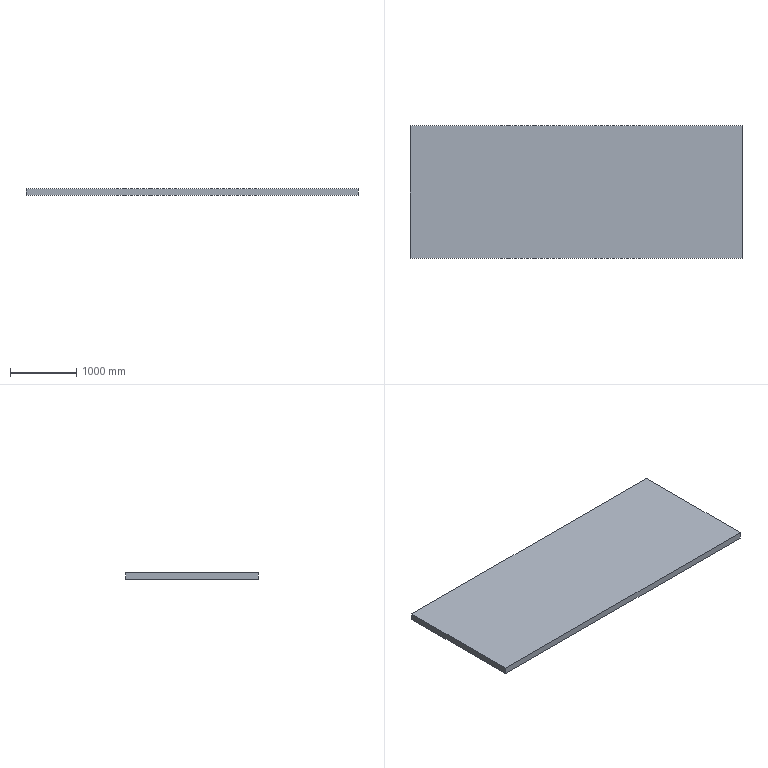Part | SolidWorks | features Extrusion 1 | 1 solid | 6 faces | box 5000 x 2000 x 100 mm | volume 1000000000 mm3 | plane 6
STEP:
#1=CARTESIAN_POINT('',(0.,2000.,0.));
#2=VERTEX_POINT('',#1);
#3=CARTESIAN_POINT('',(0.,0.,0.));
#4=VERTEX_POINT('',#3);
#5=CARTESIAN_POINT('',(0.,0.,0.));
#6=DIRECTION('',(0.,-1.,0.));
#7=VECTOR('',#6,1000.);
#8=LINE('',#5,#7);
#9=EDGE_CURVE('',#2,#4,#8,.T.);
#10=ORIENTED_EDGE('',*,*,#9,.T.);
#11=CARTESIAN_POINT('',(0.,0.,100.));
#12=VERTEX_POINT('',#11);
#13=CARTESIAN_POINT('',(0.,0.,100.));
#14=DIRECTION('',(0.,0.,-1.));
#15=VECTOR('',#14,1000.);
#16=LINE('',#13,#15);
#17=EDGE_CURVE('',#12,#4,#16,.T.);
#18=ORIENTED_EDGE('',*,*,#17,.F.);
#19=CARTESIAN_POINT('',(0.,2000.,100.));
#20=VERTEX_POINT('',#19);
#21=CARTESIAN_POINT('',(0.,0.,100.));
#22=DIRECTION('',(0.,-1.,0.));
#23=VECTOR('',#22,1000.);
#24=LINE('',#21,#23);
#25=EDGE_CURVE('',#20,#12,#24,.T.);
#26=ORIENTED_EDGE('',*,*,#25,.F.);
#27=CARTESIAN_POINT('',(0.,2000.,100.));
#28=DIRECTION('',(0.,0.,-1.));
#29=VECTOR('',#28,1000.);
#30=LINE('',#27,#29);
#31=EDGE_CURVE('',#20,#2,#30,.T.);
#32=ORIENTED_EDGE('',*,*,#31,.T.);
#33=EDGE_LOOP('',(#10,#18,#26,#32));
#34=FACE_OUTER_BOUND('',#33,.T.);
#35=CARTESIAN_POINT('',(0.,0.,100.));
#36=DIRECTION('',(1.,0.,0.));
#37=DIRECTION('',(0.,0.,-1.));
#38=AXIS2_PLACEMENT_3D('',#35,#36,#37);
#39=PLANE('',#38);
#40=ADVANCED_FACE('',(#34),#39,.F.);
#41=CARTESIAN_POINT('',(5000.,0.,0.));
#42=VERTEX_POINT('',#41);
#43=CARTESIAN_POINT('',(0.,0.,0.));
#44=DIRECTION('',(1.,0.,0.));
#45=VECTOR('',#44,1000.);
#46=LINE('',#43,#45);
#47=EDGE_CURVE('',#4,#42,#46,.T.);
#48=ORIENTED_EDGE('',*,*,#47,.T.);
#49=CARTESIAN_POINT('',(5000.,0.,100.));
#50=VERTEX_POINT('',#49);
#51=CARTESIAN_POINT('',(5000.,0.,100.));
#52=DIRECTION('',(0.,0.,-1.));
#53=VECTOR('',#52,1000.);
#54=LINE('',#51,#53);
#55=EDGE_CURVE('',#50,#42,#54,.T.);
#56=ORIENTED_EDGE('',*,*,#55,.F.);
#57=CARTESIAN_POINT('',(0.,0.,100.));
#58=DIRECTION('',(1.,0.,0.));
#59=VECTOR('',#58,1000.);
#60=LINE('',#57,#59);
#61=EDGE_CURVE('',#12,#50,#60,.T.);
#62=ORIENTED_EDGE('',*,*,#61,.F.);
#63=ORIENTED_EDGE('',*,*,#17,.T.);
#64=EDGE_LOOP('',(#48,#56,#62,#63));
#65=FACE_OUTER_BOUND('',#64,.T.);
#66=CARTESIAN_POINT('',(0.,0.,100.));
#67=DIRECTION('',(0.,1.,0.));
#68=DIRECTION('',(0.,0.,1.));
#69=AXIS2_PLACEMENT_3D('',#66,#67,#68);
#70=PLANE('',#69);
#71=ADVANCED_FACE('',(#65),#70,.F.);
#72=CARTESIAN_POINT('',(5000.,2000.,0.));
#73=VERTEX_POINT('',#72);
#74=CARTESIAN_POINT('',(5000.,0.,0.));
#75=DIRECTION('',(0.,1.,0.));
#76=VECTOR('',#75,1000.);
#77=LINE('',#74,#76);
#78=EDGE_CURVE('',#42,#73,#77,.T.);
#79=ORIENTED_EDGE('',*,*,#78,.T.);
#80=CARTESIAN_POINT('',(5000.,2000.,100.));
#81=VERTEX_POINT('',#80);
#82=CARTESIAN_POINT('',(5000.,2000.,100.));
#83=DIRECTION('',(0.,0.,-1.));
#84=VECTOR('',#83,1000.);
#85=LINE('',#82,#84);
#86=EDGE_CURVE('',#81,#73,#85,.T.);
#87=ORIENTED_EDGE('',*,*,#86,.F.);
#88=CARTESIAN_POINT('',(5000.,0.,100.));
#89=DIRECTION('',(0.,1.,0.));
#90=VECTOR('',#89,1000.);
#91=LINE('',#88,#90);
#92=EDGE_CURVE('',#50,#81,#91,.T.);
#93=ORIENTED_EDGE('',*,*,#92,.F.);
#94=ORIENTED_EDGE('',*,*,#55,.T.);
#95=EDGE_LOOP('',(#79,#87,#93,#94));
#96=FACE_OUTER_BOUND('',#95,.T.);
#97=CARTESIAN_POINT('',(5000.,0.,100.));
#98=DIRECTION('',(-1.,0.,0.));
#99=DIRECTION('',(0.,0.,1.));
#100=AXIS2_PLACEMENT_3D('',#97,#98,#99);
#101=PLANE('',#100);
#102=ADVANCED_FACE('',(#96),#101,.F.);
#103=CARTESIAN_POINT('',(0.,2000.,0.));
#104=DIRECTION('',(-1.,0.,0.));
#105=VECTOR('',#104,1000.);
#106=LINE('',#103,#105);
#107=EDGE_CURVE('',#73,#2,#106,.T.);
#108=ORIENTED_EDGE('',*,*,#107,.T.);
#109=ORIENTED_EDGE('',*,*,#31,.F.);
#110=CARTESIAN_POINT('',(0.,2000.,100.));
#111=DIRECTION('',(-1.,0.,0.));
#112=VECTOR('',#111,1000.);
#113=LINE('',#110,#112);
#114=EDGE_CURVE('',#81,#20,#113,.T.);
#115=ORIENTED_EDGE('',*,*,#114,.F.);
#116=ORIENTED_EDGE('',*,*,#86,.T.);
#117=EDGE_LOOP('',(#108,#109,#115,#116));
#118=FACE_OUTER_BOUND('',#117,.T.);
#119=CARTESIAN_POINT('',(0.,2000.,100.));
#120=DIRECTION('',(0.,-1.,0.));
#121=DIRECTION('',(0.,0.,-1.));
#122=AXIS2_PLACEMENT_3D('',#119,#120,#121);
#123=PLANE('',#122);
#124=ADVANCED_FACE('',(#118),#123,.F.);
#125=ORIENTED_EDGE('',*,*,#25,.T.);
#126=ORIENTED_EDGE('',*,*,#61,.T.);
#127=ORIENTED_EDGE('',*,*,#92,.T.);
#128=ORIENTED_EDGE('',*,*,#114,.T.);
#129=EDGE_LOOP('',(#125,#126,#127,#128));
#130=FACE_OUTER_BOUND('',#129,.T.);
#131=CARTESIAN_POINT('',(0.,2000.,100.));
#132=DIRECTION('',(0.,0.,-1.));
#133=DIRECTION('',(-1.,0.,0.));
#134=AXIS2_PLACEMENT_3D('',#131,#132,#133);
#135=PLANE('',#134);
#136=ADVANCED_FACE('',(#130),#135,.F.);
#137=ORIENTED_EDGE('',*,*,#9,.F.);
#138=ORIENTED_EDGE('',*,*,#107,.F.);
#139=ORIENTED_EDGE('',*,*,#78,.F.);
#140=ORIENTED_EDGE('',*,*,#47,.F.);
#141=EDGE_LOOP('',(#137,#138,#139,#140));
#142=FACE_OUTER_BOUND('',#141,.T.);
#143=CARTESIAN_POINT('',(0.,2000.,0.));
#144=DIRECTION('',(0.,0.,-1.));
#145=DIRECTION('',(-1.,0.,0.));
#146=AXIS2_PLACEMENT_3D('',#143,#144,#145);
#147=PLANE('',#146);
#148=ADVANCED_FACE('',(#142),#147,.T.);
#149=CLOSED_SHELL('',(#40,#71,#102,#124,#136,#148));
#150=MANIFOLD_SOLID_BREP('',#149);
#151=CARTESIAN_POINT('',(0.,0.,0.));
#152=DIRECTION('',(0.,0.,1.));
#153=DIRECTION('',(1.,0.,0.));
#154=AXIS2_PLACEMENT_3D('',#151,#152,#153);
#155=(LENGTH_UNIT()NAMED_UNIT(*)SI_UNIT(.MILLI.,.METRE.));
#156=UNCERTAINTY_MEASURE_WITH_UNIT(LENGTH_MEASURE(0.00001),#155,'','');
#157=(NAMED_UNIT(*)PLANE_ANGLE_UNIT()SI_UNIT($,.RADIAN.));
#158=(NAMED_UNIT(*)SI_UNIT($,.STERADIAN.)SOLID_ANGLE_UNIT());
#159=(GEOMETRIC_REPRESENTATION_CONTEXT(3)GLOBAL_UNCERTAINTY_ASSIGNED_CONTEXT((#156))GLOBAL_UNIT_ASSIGNED_CONTEXT((#155,#157,#158))REPRESENTATION_CONTEXT('',''));
#160=ADVANCED_BREP_SHAPE_REPRESENTATION('',(#150,#154),#159);